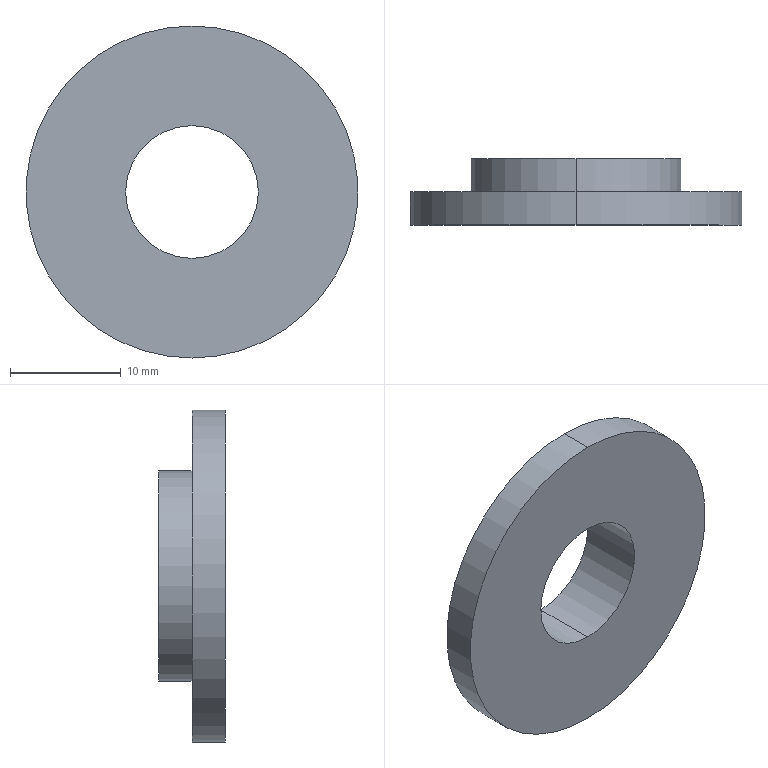Part | SolidWorks | features ICE 2, Extrusion 1 | 1 solid | 9 faces | box 30 x 6 x 30 mm | volume 2293 mm3 | cylinder 6 | plane 3 | commonest cylinder face diameters 12 x2 19 x2 30 x2
STEP:
#1=CARTESIAN_POINT('',(0.,0.,-6.));
#2=VERTEX_POINT('',#1);
#3=CARTESIAN_POINT('',(0.,0.,6.));
#4=VERTEX_POINT('',#3);
#5=CARTESIAN_POINT('',(0.,0.,0.));
#6=DIRECTION('',(0.,1.,0.));
#7=DIRECTION('',(0.,0.,1.));
#8=AXIS2_PLACEMENT_3D('',#5,#6,#7);
#9=CIRCLE('',#8,6.);
#10=EDGE_CURVE('',#2,#4,#9,.T.);
#11=ORIENTED_EDGE('',*,*,#10,.F.);
#12=CARTESIAN_POINT('',(0.,6.,-6.));
#13=VERTEX_POINT('',#12);
#14=CARTESIAN_POINT('',(0.,-4.,-6.));
#15=DIRECTION('',(0.,1.,0.));
#16=VECTOR('',#15,1000.);
#17=LINE('',#14,#16);
#18=EDGE_CURVE('',#2,#13,#17,.T.);
#19=ORIENTED_EDGE('',*,*,#18,.T.);
#20=CARTESIAN_POINT('',(0.,6.,6.));
#21=VERTEX_POINT('',#20);
#22=CARTESIAN_POINT('',(0.,6.,0.));
#23=DIRECTION('',(0.,1.,0.));
#24=DIRECTION('',(0.,0.,1.));
#25=AXIS2_PLACEMENT_3D('',#22,#23,#24);
#26=CIRCLE('',#25,6.);
#27=EDGE_CURVE('',#13,#21,#26,.T.);
#28=ORIENTED_EDGE('',*,*,#27,.T.);
#29=CARTESIAN_POINT('',(0.,-4.,6.));
#30=DIRECTION('',(0.,1.,0.));
#31=VECTOR('',#30,1000.);
#32=LINE('',#29,#31);
#33=EDGE_CURVE('',#4,#21,#32,.T.);
#34=ORIENTED_EDGE('',*,*,#33,.F.);
#35=EDGE_LOOP('',(#11,#19,#28,#34));
#36=FACE_OUTER_BOUND('',#35,.T.);
#37=CARTESIAN_POINT('',(0.,-4.,0.));
#38=DIRECTION('',(0.,1.,0.));
#39=DIRECTION('',(0.,0.,1.));
#40=AXIS2_PLACEMENT_3D('',#37,#38,#39);
#41=CYLINDRICAL_SURFACE('',#40,6.);
#42=ADVANCED_FACE('',(#36),#41,.F.);
#43=CARTESIAN_POINT('',(0.,6.,9.5));
#44=VERTEX_POINT('',#43);
#45=CARTESIAN_POINT('',(0.,6.,-9.5));
#46=VERTEX_POINT('',#45);
#47=CARTESIAN_POINT('',(0.,6.,0.));
#48=DIRECTION('',(0.,1.,0.));
#49=DIRECTION('',(0.,0.,1.));
#50=AXIS2_PLACEMENT_3D('',#47,#48,#49);
#51=CIRCLE('',#50,9.5);
#52=EDGE_CURVE('',#44,#46,#51,.T.);
#53=ORIENTED_EDGE('',*,*,#52,.F.);
#54=CARTESIAN_POINT('',(0.,3.,9.5));
#55=VERTEX_POINT('',#54);
#56=CARTESIAN_POINT('',(0.,6.,9.5));
#57=DIRECTION('',(0.,-1.,0.));
#58=VECTOR('',#57,1000.);
#59=LINE('',#56,#58);
#60=EDGE_CURVE('',#44,#55,#59,.T.);
#61=ORIENTED_EDGE('',*,*,#60,.T.);
#62=CARTESIAN_POINT('',(0.,3.,-9.5));
#63=VERTEX_POINT('',#62);
#64=CARTESIAN_POINT('',(0.,3.,0.));
#65=DIRECTION('',(0.,1.,0.));
#66=DIRECTION('',(0.,0.,1.));
#67=AXIS2_PLACEMENT_3D('',#64,#65,#66);
#68=CIRCLE('',#67,9.5);
#69=EDGE_CURVE('',#55,#63,#68,.T.);
#70=ORIENTED_EDGE('',*,*,#69,.T.);
#71=CARTESIAN_POINT('',(0.,6.,-9.5));
#72=DIRECTION('',(0.,-1.,0.));
#73=VECTOR('',#72,1000.);
#74=LINE('',#71,#73);
#75=EDGE_CURVE('',#46,#63,#74,.T.);
#76=ORIENTED_EDGE('',*,*,#75,.F.);
#77=EDGE_LOOP('',(#53,#61,#70,#76));
#78=FACE_OUTER_BOUND('',#77,.T.);
#79=CARTESIAN_POINT('',(0.,6.,0.));
#80=DIRECTION('',(0.,-1.,0.));
#81=DIRECTION('',(0.,0.,-1.));
#82=AXIS2_PLACEMENT_3D('',#79,#80,#81);
#83=CYLINDRICAL_SURFACE('',#82,9.5);
#84=ADVANCED_FACE('',(#78),#83,.T.);
#85=CARTESIAN_POINT('',(0.,3.,15.));
#86=VERTEX_POINT('',#85);
#87=CARTESIAN_POINT('',(0.,3.,-15.));
#88=VERTEX_POINT('',#87);
#89=CARTESIAN_POINT('',(0.,3.,0.));
#90=DIRECTION('',(0.,1.,0.));
#91=DIRECTION('',(0.,0.,1.));
#92=AXIS2_PLACEMENT_3D('',#89,#90,#91);
#93=CIRCLE('',#92,15.);
#94=EDGE_CURVE('',#86,#88,#93,.T.);
#95=ORIENTED_EDGE('',*,*,#94,.F.);
#96=CARTESIAN_POINT('',(0.,0.,15.));
#97=VERTEX_POINT('',#96);
#98=CARTESIAN_POINT('',(0.,3.,15.));
#99=DIRECTION('',(0.,-1.,0.));
#100=VECTOR('',#99,1000.);
#101=LINE('',#98,#100);
#102=EDGE_CURVE('',#86,#97,#101,.T.);
#103=ORIENTED_EDGE('',*,*,#102,.T.);
#104=CARTESIAN_POINT('',(0.,0.,-15.));
#105=VERTEX_POINT('',#104);
#106=CARTESIAN_POINT('',(0.,0.,0.));
#107=DIRECTION('',(0.,1.,0.));
#108=DIRECTION('',(0.,0.,1.));
#109=AXIS2_PLACEMENT_3D('',#106,#107,#108);
#110=CIRCLE('',#109,15.);
#111=EDGE_CURVE('',#97,#105,#110,.T.);
#112=ORIENTED_EDGE('',*,*,#111,.T.);
#113=CARTESIAN_POINT('',(0.,3.,-15.));
#114=DIRECTION('',(0.,-1.,0.));
#115=VECTOR('',#114,1000.);
#116=LINE('',#113,#115);
#117=EDGE_CURVE('',#88,#105,#116,.T.);
#118=ORIENTED_EDGE('',*,*,#117,.F.);
#119=EDGE_LOOP('',(#95,#103,#112,#118));
#120=FACE_OUTER_BOUND('',#119,.T.);
#121=CARTESIAN_POINT('',(0.,3.,0.));
#122=DIRECTION('',(0.,-1.,0.));
#123=DIRECTION('',(0.,0.,-1.));
#124=AXIS2_PLACEMENT_3D('',#121,#122,#123);
#125=CYLINDRICAL_SURFACE('',#124,15.);
#126=ADVANCED_FACE('',(#120),#125,.T.);
#127=ORIENTED_EDGE('',*,*,#102,.F.);
#128=CARTESIAN_POINT('',(0.,3.,0.));
#129=DIRECTION('',(0.,1.,0.));
#130=DIRECTION('',(0.,0.,1.));
#131=AXIS2_PLACEMENT_3D('',#128,#129,#130);
#132=CIRCLE('',#131,15.);
#133=EDGE_CURVE('',#88,#86,#132,.T.);
#134=ORIENTED_EDGE('',*,*,#133,.F.);
#135=ORIENTED_EDGE('',*,*,#117,.T.);
#136=CARTESIAN_POINT('',(0.,0.,0.));
#137=DIRECTION('',(0.,1.,0.));
#138=DIRECTION('',(0.,0.,1.));
#139=AXIS2_PLACEMENT_3D('',#136,#137,#138);
#140=CIRCLE('',#139,15.);
#141=EDGE_CURVE('',#105,#97,#140,.T.);
#142=ORIENTED_EDGE('',*,*,#141,.T.);
#143=EDGE_LOOP('',(#127,#134,#135,#142));
#144=FACE_OUTER_BOUND('',#143,.T.);
#145=CARTESIAN_POINT('',(0.,3.,0.));
#146=DIRECTION('',(0.,-1.,0.));
#147=DIRECTION('',(0.,0.,-1.));
#148=AXIS2_PLACEMENT_3D('',#145,#146,#147);
#149=CYLINDRICAL_SURFACE('',#148,15.);
#150=ADVANCED_FACE('',(#144),#149,.T.);
#151=CARTESIAN_POINT('',(0.,3.,0.));
#152=DIRECTION('',(0.,1.,0.));
#153=DIRECTION('',(0.,0.,1.));
#154=AXIS2_PLACEMENT_3D('',#151,#152,#153);
#155=CIRCLE('',#154,9.5);
#156=EDGE_CURVE('',#63,#55,#155,.T.);
#157=ORIENTED_EDGE('',*,*,#156,.F.);
#158=ORIENTED_EDGE('',*,*,#69,.F.);
#159=EDGE_LOOP('',(#157,#158));
#160=FACE_BOUND('',#159,.T.);
#161=ORIENTED_EDGE('',*,*,#133,.T.);
#162=ORIENTED_EDGE('',*,*,#94,.T.);
#163=EDGE_LOOP('',(#161,#162));
#164=FACE_OUTER_BOUND('',#163,.T.);
#165=CARTESIAN_POINT('',(0.,3.,0.));
#166=DIRECTION('',(0.,1.,0.));
#167=DIRECTION('',(0.,0.,1.));
#168=AXIS2_PLACEMENT_3D('',#165,#166,#167);
#169=PLANE('',#168);
#170=ADVANCED_FACE('',(#160,#164),#169,.T.);
#171=CARTESIAN_POINT('',(0.,0.,0.));
#172=DIRECTION('',(0.,1.,0.));
#173=DIRECTION('',(0.,0.,1.));
#174=AXIS2_PLACEMENT_3D('',#171,#172,#173);
#175=CIRCLE('',#174,6.);
#176=EDGE_CURVE('',#4,#2,#175,.T.);
#177=ORIENTED_EDGE('',*,*,#176,.T.);
#178=ORIENTED_EDGE('',*,*,#10,.T.);
#179=EDGE_LOOP('',(#177,#178));
#180=FACE_BOUND('',#179,.T.);
#181=ORIENTED_EDGE('',*,*,#141,.F.);
#182=ORIENTED_EDGE('',*,*,#111,.F.);
#183=EDGE_LOOP('',(#181,#182));
#184=FACE_OUTER_BOUND('',#183,.T.);
#185=CARTESIAN_POINT('',(0.,0.,0.));
#186=DIRECTION('',(0.,1.,0.));
#187=DIRECTION('',(0.,0.,1.));
#188=AXIS2_PLACEMENT_3D('',#185,#186,#187);
#189=PLANE('',#188);
#190=ADVANCED_FACE('',(#180,#184),#189,.F.);
#191=ORIENTED_EDGE('',*,*,#60,.F.);
#192=CARTESIAN_POINT('',(0.,6.,0.));
#193=DIRECTION('',(0.,1.,0.));
#194=DIRECTION('',(0.,0.,1.));
#195=AXIS2_PLACEMENT_3D('',#192,#193,#194);
#196=CIRCLE('',#195,9.5);
#197=EDGE_CURVE('',#46,#44,#196,.T.);
#198=ORIENTED_EDGE('',*,*,#197,.F.);
#199=ORIENTED_EDGE('',*,*,#75,.T.);
#200=ORIENTED_EDGE('',*,*,#156,.T.);
#201=EDGE_LOOP('',(#191,#198,#199,#200));
#202=FACE_OUTER_BOUND('',#201,.T.);
#203=CARTESIAN_POINT('',(0.,6.,0.));
#204=DIRECTION('',(0.,-1.,0.));
#205=DIRECTION('',(0.,0.,-1.));
#206=AXIS2_PLACEMENT_3D('',#203,#204,#205);
#207=CYLINDRICAL_SURFACE('',#206,9.5);
#208=ADVANCED_FACE('',(#202),#207,.T.);
#209=CARTESIAN_POINT('',(0.,6.,0.));
#210=DIRECTION('',(0.,1.,0.));
#211=DIRECTION('',(0.,0.,1.));
#212=AXIS2_PLACEMENT_3D('',#209,#210,#211);
#213=CIRCLE('',#212,6.);
#214=EDGE_CURVE('',#21,#13,#213,.T.);
#215=ORIENTED_EDGE('',*,*,#214,.F.);
#216=ORIENTED_EDGE('',*,*,#27,.F.);
#217=EDGE_LOOP('',(#215,#216));
#218=FACE_BOUND('',#217,.T.);
#219=ORIENTED_EDGE('',*,*,#197,.T.);
#220=ORIENTED_EDGE('',*,*,#52,.T.);
#221=EDGE_LOOP('',(#219,#220));
#222=FACE_OUTER_BOUND('',#221,.T.);
#223=CARTESIAN_POINT('',(0.,6.,0.));
#224=DIRECTION('',(0.,1.,0.));
#225=DIRECTION('',(0.,0.,1.));
#226=AXIS2_PLACEMENT_3D('',#223,#224,#225);
#227=PLANE('',#226);
#228=ADVANCED_FACE('',(#218,#222),#227,.T.);
#229=ORIENTED_EDGE('',*,*,#18,.F.);
#230=ORIENTED_EDGE('',*,*,#176,.F.);
#231=ORIENTED_EDGE('',*,*,#33,.T.);
#232=ORIENTED_EDGE('',*,*,#214,.T.);
#233=EDGE_LOOP('',(#229,#230,#231,#232));
#234=FACE_OUTER_BOUND('',#233,.T.);
#235=CARTESIAN_POINT('',(0.,-4.,0.));
#236=DIRECTION('',(0.,1.,0.));
#237=DIRECTION('',(0.,0.,1.));
#238=AXIS2_PLACEMENT_3D('',#235,#236,#237);
#239=CYLINDRICAL_SURFACE('',#238,6.);
#240=ADVANCED_FACE('',(#234),#239,.F.);
#241=CLOSED_SHELL('',(#42,#84,#126,#150,#170,#190,#208,#228,#240));
#242=MANIFOLD_SOLID_BREP('',#241);
#243=CARTESIAN_POINT('',(0.,0.,0.));
#244=DIRECTION('',(0.,0.,1.));
#245=DIRECTION('',(1.,0.,0.));
#246=AXIS2_PLACEMENT_3D('',#243,#244,#245);
#247=(LENGTH_UNIT()NAMED_UNIT(*)SI_UNIT(.MILLI.,.METRE.));
#248=UNCERTAINTY_MEASURE_WITH_UNIT(LENGTH_MEASURE(0.00001),#247,'','');
#249=(NAMED_UNIT(*)PLANE_ANGLE_UNIT()SI_UNIT($,.RADIAN.));
#250=(NAMED_UNIT(*)SI_UNIT($,.STERADIAN.)SOLID_ANGLE_UNIT());
#251=(GEOMETRIC_REPRESENTATION_CONTEXT(3)GLOBAL_UNCERTAINTY_ASSIGNED_CONTEXT((#248))GLOBAL_UNIT_ASSIGNED_CONTEXT((#247,#249,#250))REPRESENTATION_CONTEXT('',''));
#252=ADVANCED_BREP_SHAPE_REPRESENTATION('',(#242,#246),#251);